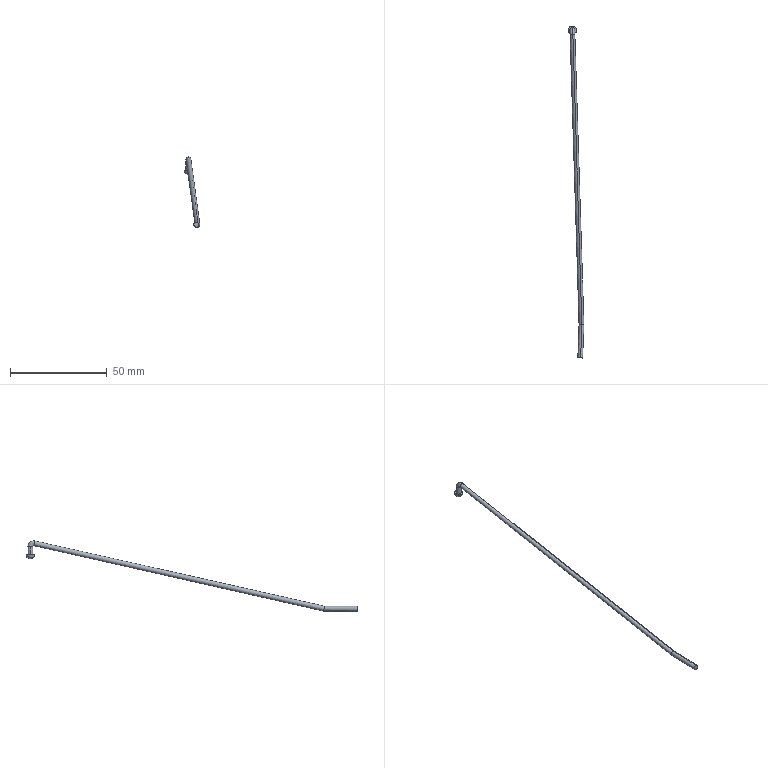Part | STEP file | Spoke_1 | 1 solid | 12 faces | box 8.143 x 171.447 x 36.243 mm | volume 895.693 mm3 | spline 6 | sphere 2 | cylinder 2 | plane 2 | commonest cylinder face diameters 2.5 x2